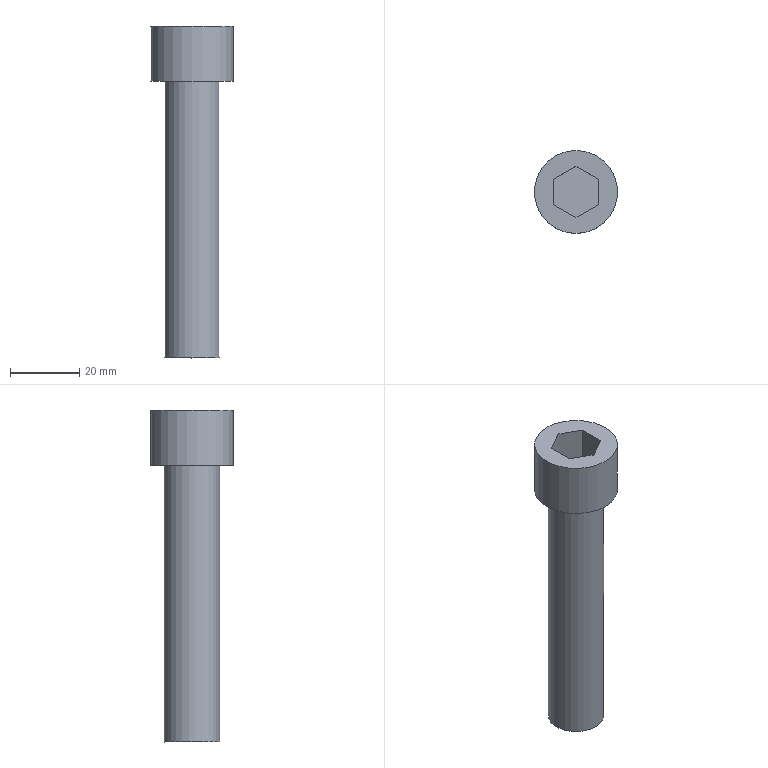Part | NX | features solid 2 | 1 solid | 12 faces | box 24 x 24 x 96 mm | volume 21961 mm3 | plane 10 | cylinder 2 | commonest cylinder face diameters 16 x1 24 x1
STEP:
#1=CARTESIAN_POINT('',(-291.4,260.695,-49.));
#2=VERTEX_POINT('',#1);
#3=CARTESIAN_POINT('',(-285.,264.39,-49.));
#4=VERTEX_POINT('',#3);
#5=CARTESIAN_POINT('',(-288.2,262.543,-49.));
#6=DIRECTION('',(0.866,0.5,0.));
#7=VECTOR('',#6,1000.);
#8=LINE('',#5,#7);
#9=EDGE_CURVE('',#2,#4,#8,.T.);
#10=ORIENTED_EDGE('',*,*,#9,.T.);
#11=CARTESIAN_POINT('',(-278.6,260.695,-49.));
#12=VERTEX_POINT('',#11);
#13=CARTESIAN_POINT('',(-281.8,262.543,-49.));
#14=DIRECTION('',(0.866,-0.5,0.));
#15=VECTOR('',#14,1000.);
#16=LINE('',#13,#15);
#17=EDGE_CURVE('',#4,#12,#16,.T.);
#18=ORIENTED_EDGE('',*,*,#17,.T.);
#19=CARTESIAN_POINT('',(-278.6,253.305,-49.));
#20=VERTEX_POINT('',#19);
#21=CARTESIAN_POINT('',(-278.6,257.,-49.));
#22=DIRECTION('',(0.,-1.,0.));
#23=VECTOR('',#22,1000.);
#24=LINE('',#21,#23);
#25=EDGE_CURVE('',#12,#20,#24,.T.);
#26=ORIENTED_EDGE('',*,*,#25,.T.);
#27=CARTESIAN_POINT('',(-285.,249.61,-49.));
#28=VERTEX_POINT('',#27);
#29=CARTESIAN_POINT('',(-281.8,251.457,-49.));
#30=DIRECTION('',(-0.866,-0.5,0.));
#31=VECTOR('',#30,1000.);
#32=LINE('',#29,#31);
#33=EDGE_CURVE('',#20,#28,#32,.T.);
#34=ORIENTED_EDGE('',*,*,#33,.T.);
#35=CARTESIAN_POINT('',(-291.4,253.305,-49.));
#36=VERTEX_POINT('',#35);
#37=CARTESIAN_POINT('',(-288.2,251.457,-49.));
#38=DIRECTION('',(-0.866,0.5,0.));
#39=VECTOR('',#38,1000.);
#40=LINE('',#37,#39);
#41=EDGE_CURVE('',#28,#36,#40,.T.);
#42=ORIENTED_EDGE('',*,*,#41,.T.);
#43=CARTESIAN_POINT('',(-291.4,257.,-49.));
#44=DIRECTION('',(0.,1.,0.));
#45=VECTOR('',#44,1000.);
#46=LINE('',#43,#45);
#47=EDGE_CURVE('',#36,#2,#46,.T.);
#48=ORIENTED_EDGE('',*,*,#47,.T.);
#49=EDGE_LOOP('',(#10,#18,#26,#34,#42,#48));
#50=FACE_BOUND('',#49,.T.);
#51=CARTESIAN_POINT('',(-285.,269.,-49.));
#52=VERTEX_POINT('',#51);
#53=CARTESIAN_POINT('',(-285.,257.,-49.));
#54=DIRECTION('',(0.,0.,1.));
#55=DIRECTION('',(0.,1.,0.));
#56=AXIS2_PLACEMENT_3D('',#53,#54,#55);
#57=CIRCLE('',#56,12.);
#58=EDGE_CURVE('',#52,#52,#57,.T.);
#59=ORIENTED_EDGE('',*,*,#58,.T.);
#60=EDGE_LOOP('',(#59));
#61=FACE_BOUND('',#60,.T.);
#62=CARTESIAN_POINT('',(-285.,257.,-49.));
#63=DIRECTION('',(0.,0.,1.));
#64=DIRECTION('',(0.,-1.,0.));
#65=AXIS2_PLACEMENT_3D('',#62,#63,#64);
#66=PLANE('',#65);
#67=ADVANCED_FACE('',(#50,#61),#66,.T.);
#68=CARTESIAN_POINT('',(-285.,265.,-65.));
#69=VERTEX_POINT('',#68);
#70=CARTESIAN_POINT('',(-285.,257.,-65.));
#71=DIRECTION('',(0.,0.,1.));
#72=DIRECTION('',(0.,1.,0.));
#73=AXIS2_PLACEMENT_3D('',#70,#71,#72);
#74=CIRCLE('',#73,8.);
#75=EDGE_CURVE('',#69,#69,#74,.T.);
#76=ORIENTED_EDGE('',*,*,#75,.T.);
#77=EDGE_LOOP('',(#76));
#78=FACE_BOUND('',#77,.T.);
#79=CARTESIAN_POINT('',(-285.,245.,-65.));
#80=VERTEX_POINT('',#79);
#81=CARTESIAN_POINT('',(-285.,257.,-65.));
#82=DIRECTION('',(0.,0.,-1.));
#83=DIRECTION('',(0.,-1.,0.));
#84=AXIS2_PLACEMENT_3D('',#81,#82,#83);
#85=CIRCLE('',#84,12.);
#86=EDGE_CURVE('',#80,#80,#85,.T.);
#87=ORIENTED_EDGE('',*,*,#86,.T.);
#88=EDGE_LOOP('',(#87));
#89=FACE_BOUND('',#88,.T.);
#90=CARTESIAN_POINT('',(-285.,257.,-65.));
#91=DIRECTION('',(0.,0.,-1.));
#92=DIRECTION('',(0.,1.,0.));
#93=AXIS2_PLACEMENT_3D('',#90,#91,#92);
#94=PLANE('',#93);
#95=ADVANCED_FACE('',(#78,#89),#94,.T.);
#96=ORIENTED_EDGE('',*,*,#58,.F.);
#97=EDGE_LOOP('',(#96));
#98=FACE_BOUND('',#97,.T.);
#99=ORIENTED_EDGE('',*,*,#86,.F.);
#100=EDGE_LOOP('',(#99));
#101=FACE_BOUND('',#100,.T.);
#102=CARTESIAN_POINT('',(-285.,257.,-65.));
#103=DIRECTION('',(0.,0.,1.));
#104=DIRECTION('',(0.,-1.,0.));
#105=AXIS2_PLACEMENT_3D('',#102,#103,#104);
#106=CYLINDRICAL_SURFACE('',#105,12.);
#107=ADVANCED_FACE('',(#98,#101),#106,.T.);
#108=ORIENTED_EDGE('',*,*,#9,.F.);
#109=CARTESIAN_POINT('',(-291.4,260.695,-58.6));
#110=VERTEX_POINT('',#109);
#111=CARTESIAN_POINT('',(-291.4,260.695,-58.6));
#112=DIRECTION('',(0.,0.,1.));
#113=VECTOR('',#112,1000.);
#114=LINE('',#111,#113);
#115=EDGE_CURVE('',#110,#2,#114,.T.);
#116=ORIENTED_EDGE('',*,*,#115,.F.);
#117=CARTESIAN_POINT('',(-285.,264.39,-58.6));
#118=VERTEX_POINT('',#117);
#119=CARTESIAN_POINT('',(-291.4,260.695,-58.6));
#120=DIRECTION('',(0.866,0.5,0.));
#121=VECTOR('',#120,1000.);
#122=LINE('',#119,#121);
#123=EDGE_CURVE('',#110,#118,#122,.T.);
#124=ORIENTED_EDGE('',*,*,#123,.T.);
#125=CARTESIAN_POINT('',(-285.,264.39,-58.6));
#126=DIRECTION('',(0.,0.,1.));
#127=VECTOR('',#126,1000.);
#128=LINE('',#125,#127);
#129=EDGE_CURVE('',#118,#4,#128,.T.);
#130=ORIENTED_EDGE('',*,*,#129,.T.);
#131=EDGE_LOOP('',(#108,#116,#124,#130));
#132=FACE_BOUND('',#131,.T.);
#133=CARTESIAN_POINT('',(-288.2,262.543,-50.6));
#134=DIRECTION('',(-0.5,0.866,0.));
#135=DIRECTION('',(-0.866,-0.5,0.));
#136=AXIS2_PLACEMENT_3D('',#133,#134,#135);
#137=PLANE('',#136);
#138=ADVANCED_FACE('',(#132),#137,.F.);
#139=ORIENTED_EDGE('',*,*,#47,.F.);
#140=CARTESIAN_POINT('',(-291.4,253.305,-58.6));
#141=VERTEX_POINT('',#140);
#142=CARTESIAN_POINT('',(-291.4,253.305,-58.6));
#143=DIRECTION('',(0.,0.,1.));
#144=VECTOR('',#143,1000.);
#145=LINE('',#142,#144);
#146=EDGE_CURVE('',#141,#36,#145,.T.);
#147=ORIENTED_EDGE('',*,*,#146,.F.);
#148=CARTESIAN_POINT('',(-291.4,253.305,-58.6));
#149=DIRECTION('',(0.,1.,0.));
#150=VECTOR('',#149,1000.);
#151=LINE('',#148,#150);
#152=EDGE_CURVE('',#141,#110,#151,.T.);
#153=ORIENTED_EDGE('',*,*,#152,.T.);
#154=ORIENTED_EDGE('',*,*,#115,.T.);
#155=EDGE_LOOP('',(#139,#147,#153,#154));
#156=FACE_BOUND('',#155,.T.);
#157=CARTESIAN_POINT('',(-291.4,257.,-50.6));
#158=DIRECTION('',(-1.,0.,0.));
#159=DIRECTION('',(0.,-1.,0.));
#160=AXIS2_PLACEMENT_3D('',#157,#158,#159);
#161=PLANE('',#160);
#162=ADVANCED_FACE('',(#156),#161,.F.);
#163=ORIENTED_EDGE('',*,*,#41,.F.);
#164=CARTESIAN_POINT('',(-285.,249.61,-58.6));
#165=VERTEX_POINT('',#164);
#166=CARTESIAN_POINT('',(-285.,249.61,-58.6));
#167=DIRECTION('',(0.,0.,1.));
#168=VECTOR('',#167,1000.);
#169=LINE('',#166,#168);
#170=EDGE_CURVE('',#165,#28,#169,.T.);
#171=ORIENTED_EDGE('',*,*,#170,.F.);
#172=CARTESIAN_POINT('',(-285.,249.61,-58.6));
#173=DIRECTION('',(-0.866,0.5,0.));
#174=VECTOR('',#173,1000.);
#175=LINE('',#172,#174);
#176=EDGE_CURVE('',#165,#141,#175,.T.);
#177=ORIENTED_EDGE('',*,*,#176,.T.);
#178=ORIENTED_EDGE('',*,*,#146,.T.);
#179=EDGE_LOOP('',(#163,#171,#177,#178));
#180=FACE_BOUND('',#179,.T.);
#181=CARTESIAN_POINT('',(-288.2,251.457,-50.6));
#182=DIRECTION('',(-0.5,-0.866,0.));
#183=DIRECTION('',(0.866,-0.5,0.));
#184=AXIS2_PLACEMENT_3D('',#181,#182,#183);
#185=PLANE('',#184);
#186=ADVANCED_FACE('',(#180),#185,.F.);
#187=ORIENTED_EDGE('',*,*,#33,.F.);
#188=CARTESIAN_POINT('',(-278.6,253.305,-58.6));
#189=VERTEX_POINT('',#188);
#190=CARTESIAN_POINT('',(-278.6,253.305,-58.6));
#191=DIRECTION('',(0.,0.,1.));
#192=VECTOR('',#191,1000.);
#193=LINE('',#190,#192);
#194=EDGE_CURVE('',#189,#20,#193,.T.);
#195=ORIENTED_EDGE('',*,*,#194,.F.);
#196=CARTESIAN_POINT('',(-278.6,253.305,-58.6));
#197=DIRECTION('',(-0.866,-0.5,0.));
#198=VECTOR('',#197,1000.);
#199=LINE('',#196,#198);
#200=EDGE_CURVE('',#189,#165,#199,.T.);
#201=ORIENTED_EDGE('',*,*,#200,.T.);
#202=ORIENTED_EDGE('',*,*,#170,.T.);
#203=EDGE_LOOP('',(#187,#195,#201,#202));
#204=FACE_BOUND('',#203,.T.);
#205=CARTESIAN_POINT('',(-281.8,251.457,-50.6));
#206=DIRECTION('',(0.5,-0.866,0.));
#207=DIRECTION('',(0.866,0.5,0.));
#208=AXIS2_PLACEMENT_3D('',#205,#206,#207);
#209=PLANE('',#208);
#210=ADVANCED_FACE('',(#204),#209,.F.);
#211=ORIENTED_EDGE('',*,*,#25,.F.);
#212=CARTESIAN_POINT('',(-278.6,260.695,-58.6));
#213=VERTEX_POINT('',#212);
#214=CARTESIAN_POINT('',(-278.6,260.695,-58.6));
#215=DIRECTION('',(0.,0.,1.));
#216=VECTOR('',#215,1000.);
#217=LINE('',#214,#216);
#218=EDGE_CURVE('',#213,#12,#217,.T.);
#219=ORIENTED_EDGE('',*,*,#218,.F.);
#220=CARTESIAN_POINT('',(-278.6,260.695,-58.6));
#221=DIRECTION('',(0.,-1.,0.));
#222=VECTOR('',#221,1000.);
#223=LINE('',#220,#222);
#224=EDGE_CURVE('',#213,#189,#223,.T.);
#225=ORIENTED_EDGE('',*,*,#224,.T.);
#226=ORIENTED_EDGE('',*,*,#194,.T.);
#227=EDGE_LOOP('',(#211,#219,#225,#226));
#228=FACE_BOUND('',#227,.T.);
#229=CARTESIAN_POINT('',(-278.6,257.,-50.6));
#230=DIRECTION('',(1.,0.,0.));
#231=DIRECTION('',(0.,1.,0.));
#232=AXIS2_PLACEMENT_3D('',#229,#230,#231);
#233=PLANE('',#232);
#234=ADVANCED_FACE('',(#228),#233,.F.);
#235=ORIENTED_EDGE('',*,*,#17,.F.);
#236=ORIENTED_EDGE('',*,*,#129,.F.);
#237=CARTESIAN_POINT('',(-285.,264.39,-58.6));
#238=DIRECTION('',(0.866,-0.5,0.));
#239=VECTOR('',#238,1000.);
#240=LINE('',#237,#239);
#241=EDGE_CURVE('',#118,#213,#240,.T.);
#242=ORIENTED_EDGE('',*,*,#241,.T.);
#243=ORIENTED_EDGE('',*,*,#218,.T.);
#244=EDGE_LOOP('',(#235,#236,#242,#243));
#245=FACE_BOUND('',#244,.T.);
#246=CARTESIAN_POINT('',(-281.8,262.543,-50.6));
#247=DIRECTION('',(0.5,0.866,0.));
#248=DIRECTION('',(-0.866,0.5,0.));
#249=AXIS2_PLACEMENT_3D('',#246,#247,#248);
#250=PLANE('',#249);
#251=ADVANCED_FACE('',(#245),#250,.F.);
#252=ORIENTED_EDGE('',*,*,#241,.F.);
#253=ORIENTED_EDGE('',*,*,#123,.F.);
#254=ORIENTED_EDGE('',*,*,#152,.F.);
#255=ORIENTED_EDGE('',*,*,#176,.F.);
#256=ORIENTED_EDGE('',*,*,#200,.F.);
#257=ORIENTED_EDGE('',*,*,#224,.F.);
#258=EDGE_LOOP('',(#252,#253,#254,#255,#256,#257));
#259=FACE_BOUND('',#258,.T.);
#260=CARTESIAN_POINT('',(-285.,257.,-58.6));
#261=DIRECTION('',(0.,0.,-1.));
#262=DIRECTION('',(0.,1.,0.));
#263=AXIS2_PLACEMENT_3D('',#260,#261,#262);
#264=PLANE('',#263);
#265=ADVANCED_FACE('',(#259),#264,.F.);
#266=CARTESIAN_POINT('',(-285.,249.,-145.));
#267=VERTEX_POINT('',#266);
#268=CARTESIAN_POINT('',(-285.,257.,-145.));
#269=DIRECTION('',(0.,0.,-1.));
#270=DIRECTION('',(0.,-1.,0.));
#271=AXIS2_PLACEMENT_3D('',#268,#269,#270);
#272=CIRCLE('',#271,8.);
#273=EDGE_CURVE('',#267,#267,#272,.T.);
#274=ORIENTED_EDGE('',*,*,#273,.T.);
#275=EDGE_LOOP('',(#274));
#276=FACE_BOUND('',#275,.T.);
#277=CARTESIAN_POINT('',(-285.,257.,-145.));
#278=DIRECTION('',(0.,0.,-1.));
#279=DIRECTION('',(0.,1.,0.));
#280=AXIS2_PLACEMENT_3D('',#277,#278,#279);
#281=PLANE('',#280);
#282=ADVANCED_FACE('',(#276),#281,.T.);
#283=ORIENTED_EDGE('',*,*,#273,.F.);
#284=EDGE_LOOP('',(#283));
#285=FACE_BOUND('',#284,.T.);
#286=ORIENTED_EDGE('',*,*,#75,.F.);
#287=EDGE_LOOP('',(#286));
#288=FACE_BOUND('',#287,.T.);
#289=CARTESIAN_POINT('',(-285.,257.,-65.));
#290=DIRECTION('',(0.,0.,-1.));
#291=DIRECTION('',(0.,1.,0.));
#292=AXIS2_PLACEMENT_3D('',#289,#290,#291);
#293=CYLINDRICAL_SURFACE('',#292,8.);
#294=ADVANCED_FACE('',(#285,#288),#293,.T.);
#295=CLOSED_SHELL('',(#67,#95,#107,#138,#162,#186,#210,#234,#251,#265,#282,#294));
#296=MANIFOLD_SOLID_BREP('',#295);
#297=(LENGTH_UNIT()NAMED_UNIT(*)SI_UNIT(.MILLI.,.METRE.));
#298=UNCERTAINTY_MEASURE_WITH_UNIT(LENGTH_MEASURE(0.00001),#297,'','');
#299=(NAMED_UNIT(*)PLANE_ANGLE_UNIT()SI_UNIT($,.RADIAN.));
#300=(NAMED_UNIT(*)SI_UNIT($,.STERADIAN.)SOLID_ANGLE_UNIT());
#301=(GEOMETRIC_REPRESENTATION_CONTEXT(3)GLOBAL_UNCERTAINTY_ASSIGNED_CONTEXT((#298))GLOBAL_UNIT_ASSIGNED_CONTEXT((#297,#299,#300))REPRESENTATION_CONTEXT('',''));
#302=ADVANCED_BREP_SHAPE_REPRESENTATION('',(#296),#301);